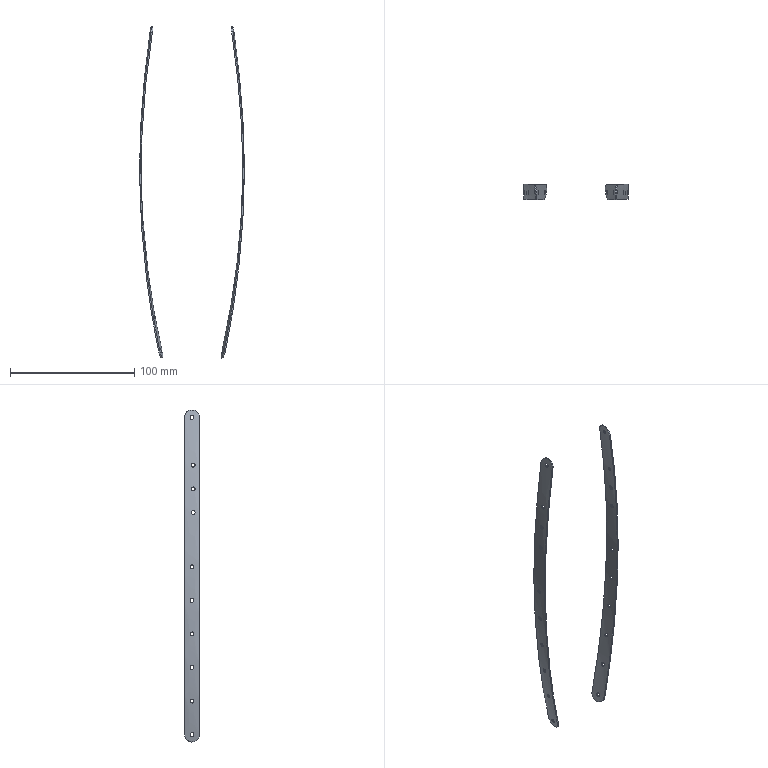Part | SolidWorks | features BaseBody 2 | 2 solids | 54 faces | box 83.978 x 12 x 267.283 mm | volume 6239 mm3 | cylinder 44 | spline 6 | plane 4 | commonest cylinder face diameters 3.2 x40 12 x4